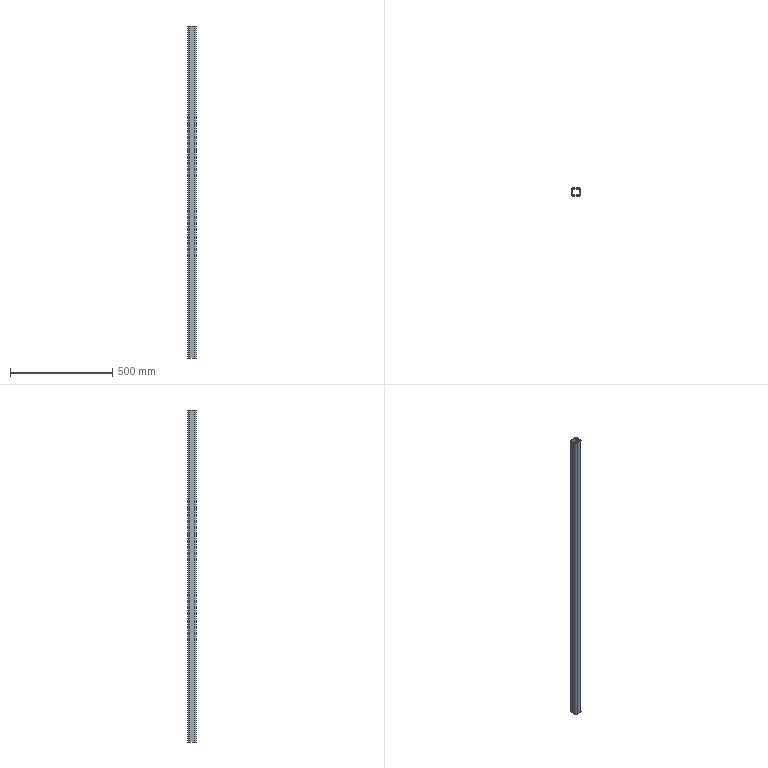Part | STEP file | 40 x 40 x 1700 | 1 solid | 18 faces | box 40 x 40 x 1620 mm | volume 866370 mm3 | plane 10 | cylinder 8 | commonest cylinder face diameters 8 x4 16 x4
STEP:
#1=CARTESIAN_POINT('',(32.,40.,1020.));
#2=VERTEX_POINT('',#1);
#3=CARTESIAN_POINT('',(8.,40.,1020.));
#4=VERTEX_POINT('',#3);
#5=CARTESIAN_POINT('',(32.,40.,1020.));
#6=DIRECTION('',(-1.,0.,0.));
#7=VECTOR('',#6,1000.);
#8=LINE('',#5,#7);
#9=EDGE_CURVE('',#2,#4,#8,.T.);
#10=ORIENTED_EDGE('',*,*,#9,.F.);
#11=CARTESIAN_POINT('',(32.,40.,-600.));
#12=VERTEX_POINT('',#11);
#13=CARTESIAN_POINT('',(32.,40.,600.));
#14=DIRECTION('',(0.,0.,1.));
#15=VECTOR('',#14,1000.);
#16=LINE('',#13,#15);
#17=EDGE_CURVE('',#12,#2,#16,.T.);
#18=ORIENTED_EDGE('',*,*,#17,.F.);
#19=CARTESIAN_POINT('',(8.,40.,-600.));
#20=VERTEX_POINT('',#19);
#21=CARTESIAN_POINT('',(32.,40.,-600.));
#22=DIRECTION('',(1.,0.,0.));
#23=VECTOR('',#22,1000.);
#24=LINE('',#21,#23);
#25=EDGE_CURVE('',#20,#12,#24,.T.);
#26=ORIENTED_EDGE('',*,*,#25,.F.);
#27=CARTESIAN_POINT('',(8.,40.,600.));
#28=DIRECTION('',(0.,0.,-1.));
#29=VECTOR('',#28,1000.);
#30=LINE('',#27,#29);
#31=EDGE_CURVE('',#4,#20,#30,.T.);
#32=ORIENTED_EDGE('',*,*,#31,.F.);
#33=EDGE_LOOP('',(#10,#18,#26,#32));
#34=FACE_OUTER_BOUND('',#33,.T.);
#35=CARTESIAN_POINT('',(32.,40.,600.));
#36=DIRECTION('',(0.,-1.,0.));
#37=DIRECTION('',(1.,0.,0.));
#38=AXIS2_PLACEMENT_3D('',#35,#36,#37);
#39=PLANE('',#38);
#40=ADVANCED_FACE('',(#34),#39,.F.);
#41=ORIENTED_EDGE('',*,*,#31,.T.);
#42=CARTESIAN_POINT('',(0.,32.,-600.));
#43=VERTEX_POINT('',#42);
#44=CARTESIAN_POINT('',(8.,32.,-600.));
#45=DIRECTION('',(0.,0.,1.));
#46=DIRECTION('',(-1.,0.,0.));
#47=AXIS2_PLACEMENT_3D('',#44,#45,#46);
#48=CIRCLE('',#47,8.);
#49=EDGE_CURVE('',#20,#43,#48,.T.);
#50=ORIENTED_EDGE('',*,*,#49,.T.);
#51=CARTESIAN_POINT('',(0.,32.,1020.));
#52=VERTEX_POINT('',#51);
#53=CARTESIAN_POINT('',(0.,32.,600.));
#54=DIRECTION('',(0.,0.,1.));
#55=VECTOR('',#54,1000.);
#56=LINE('',#53,#55);
#57=EDGE_CURVE('',#43,#52,#56,.T.);
#58=ORIENTED_EDGE('',*,*,#57,.T.);
#59=CARTESIAN_POINT('',(8.,32.,1020.));
#60=DIRECTION('',(0.,0.,-1.));
#61=DIRECTION('',(-1.,0.,0.));
#62=AXIS2_PLACEMENT_3D('',#59,#60,#61);
#63=CIRCLE('',#62,8.);
#64=EDGE_CURVE('',#52,#4,#63,.T.);
#65=ORIENTED_EDGE('',*,*,#64,.T.);
#66=EDGE_LOOP('',(#41,#50,#58,#65));
#67=FACE_OUTER_BOUND('',#66,.T.);
#68=CARTESIAN_POINT('',(8.,32.,600.));
#69=DIRECTION('',(0.,0.,-1.));
#70=DIRECTION('',(-1.,0.,0.));
#71=AXIS2_PLACEMENT_3D('',#68,#69,#70);
#72=CYLINDRICAL_SURFACE('',#71,8.);
#73=ADVANCED_FACE('',(#67),#72,.T.);
#74=CARTESIAN_POINT('',(8.,36.,1020.));
#75=VERTEX_POINT('',#74);
#76=CARTESIAN_POINT('',(32.,36.,1020.));
#77=VERTEX_POINT('',#76);
#78=CARTESIAN_POINT('',(32.,36.,1020.));
#79=DIRECTION('',(1.,0.,0.));
#80=VECTOR('',#79,1000.);
#81=LINE('',#78,#80);
#82=EDGE_CURVE('',#75,#77,#81,.T.);
#83=ORIENTED_EDGE('',*,*,#82,.T.);
#84=CARTESIAN_POINT('',(36.,32.,1020.));
#85=VERTEX_POINT('',#84);
#86=CARTESIAN_POINT('',(32.,32.,1020.));
#87=DIRECTION('',(0.,0.,-1.));
#88=DIRECTION('',(-1.,0.,0.));
#89=AXIS2_PLACEMENT_3D('',#86,#87,#88);
#90=CIRCLE('',#89,4.);
#91=EDGE_CURVE('',#77,#85,#90,.T.);
#92=ORIENTED_EDGE('',*,*,#91,.T.);
#93=CARTESIAN_POINT('',(36.,8.,1020.));
#94=VERTEX_POINT('',#93);
#95=CARTESIAN_POINT('',(36.,8.,1020.));
#96=DIRECTION('',(0.,-1.,0.));
#97=VECTOR('',#96,1000.);
#98=LINE('',#95,#97);
#99=EDGE_CURVE('',#85,#94,#98,.T.);
#100=ORIENTED_EDGE('',*,*,#99,.T.);
#101=CARTESIAN_POINT('',(32.,4.,1020.));
#102=VERTEX_POINT('',#101);
#103=CARTESIAN_POINT('',(32.,8.,1020.));
#104=DIRECTION('',(0.,0.,-1.));
#105=DIRECTION('',(-1.,0.,0.));
#106=AXIS2_PLACEMENT_3D('',#103,#104,#105);
#107=CIRCLE('',#106,4.);
#108=EDGE_CURVE('',#94,#102,#107,.T.);
#109=ORIENTED_EDGE('',*,*,#108,.T.);
#110=CARTESIAN_POINT('',(8.,4.,1020.));
#111=VERTEX_POINT('',#110);
#112=CARTESIAN_POINT('',(32.,4.,1020.));
#113=DIRECTION('',(-1.,0.,0.));
#114=VECTOR('',#113,1000.);
#115=LINE('',#112,#114);
#116=EDGE_CURVE('',#102,#111,#115,.T.);
#117=ORIENTED_EDGE('',*,*,#116,.T.);
#118=CARTESIAN_POINT('',(4.,8.,1020.));
#119=VERTEX_POINT('',#118);
#120=CARTESIAN_POINT('',(8.,8.,1020.));
#121=DIRECTION('',(0.,0.,-1.));
#122=DIRECTION('',(-1.,0.,0.));
#123=AXIS2_PLACEMENT_3D('',#120,#121,#122);
#124=CIRCLE('',#123,4.);
#125=EDGE_CURVE('',#111,#119,#124,.T.);
#126=ORIENTED_EDGE('',*,*,#125,.T.);
#127=CARTESIAN_POINT('',(4.,32.,1020.));
#128=VERTEX_POINT('',#127);
#129=CARTESIAN_POINT('',(4.,8.,1020.));
#130=DIRECTION('',(0.,1.,0.));
#131=VECTOR('',#130,1000.);
#132=LINE('',#129,#131);
#133=EDGE_CURVE('',#119,#128,#132,.T.);
#134=ORIENTED_EDGE('',*,*,#133,.T.);
#135=CARTESIAN_POINT('',(8.,32.,1020.));
#136=DIRECTION('',(0.,0.,-1.));
#137=DIRECTION('',(-1.,0.,0.));
#138=AXIS2_PLACEMENT_3D('',#135,#136,#137);
#139=CIRCLE('',#138,4.);
#140=EDGE_CURVE('',#128,#75,#139,.T.);
#141=ORIENTED_EDGE('',*,*,#140,.T.);
#142=EDGE_LOOP('',(#83,#92,#100,#109,#117,#126,#134,#141));
#143=FACE_BOUND('',#142,.T.);
#144=CARTESIAN_POINT('',(0.,8.,1020.));
#145=VERTEX_POINT('',#144);
#146=CARTESIAN_POINT('',(8.,0.,1020.));
#147=VERTEX_POINT('',#146);
#148=CARTESIAN_POINT('',(8.,8.,1020.));
#149=DIRECTION('',(0.,0.,1.));
#150=DIRECTION('',(-1.,0.,0.));
#151=AXIS2_PLACEMENT_3D('',#148,#149,#150);
#152=CIRCLE('',#151,8.);
#153=EDGE_CURVE('',#145,#147,#152,.T.);
#154=ORIENTED_EDGE('',*,*,#153,.T.);
#155=CARTESIAN_POINT('',(32.,0.,1020.));
#156=VERTEX_POINT('',#155);
#157=CARTESIAN_POINT('',(32.,0.,1020.));
#158=DIRECTION('',(1.,0.,0.));
#159=VECTOR('',#158,1000.);
#160=LINE('',#157,#159);
#161=EDGE_CURVE('',#147,#156,#160,.T.);
#162=ORIENTED_EDGE('',*,*,#161,.T.);
#163=CARTESIAN_POINT('',(40.,8.,1020.));
#164=VERTEX_POINT('',#163);
#165=CARTESIAN_POINT('',(32.,8.,1020.));
#166=DIRECTION('',(0.,0.,1.));
#167=DIRECTION('',(-1.,0.,0.));
#168=AXIS2_PLACEMENT_3D('',#165,#166,#167);
#169=CIRCLE('',#168,8.);
#170=EDGE_CURVE('',#156,#164,#169,.T.);
#171=ORIENTED_EDGE('',*,*,#170,.T.);
#172=CARTESIAN_POINT('',(40.,32.,1020.));
#173=VERTEX_POINT('',#172);
#174=CARTESIAN_POINT('',(40.,8.,1020.));
#175=DIRECTION('',(0.,1.,0.));
#176=VECTOR('',#175,1000.);
#177=LINE('',#174,#176);
#178=EDGE_CURVE('',#164,#173,#177,.T.);
#179=ORIENTED_EDGE('',*,*,#178,.T.);
#180=CARTESIAN_POINT('',(32.,32.,1020.));
#181=DIRECTION('',(0.,0.,1.));
#182=DIRECTION('',(-1.,0.,0.));
#183=AXIS2_PLACEMENT_3D('',#180,#181,#182);
#184=CIRCLE('',#183,8.);
#185=EDGE_CURVE('',#173,#2,#184,.T.);
#186=ORIENTED_EDGE('',*,*,#185,.T.);
#187=ORIENTED_EDGE('',*,*,#9,.T.);
#188=ORIENTED_EDGE('',*,*,#64,.F.);
#189=CARTESIAN_POINT('',(0.,8.,1020.));
#190=DIRECTION('',(0.,-1.,0.));
#191=VECTOR('',#190,1000.);
#192=LINE('',#189,#191);
#193=EDGE_CURVE('',#52,#145,#192,.T.);
#194=ORIENTED_EDGE('',*,*,#193,.T.);
#195=EDGE_LOOP('',(#154,#162,#171,#179,#186,#187,#188,#194));
#196=FACE_OUTER_BOUND('',#195,.T.);
#197=CARTESIAN_POINT('',(32.,8.,1020.));
#198=DIRECTION('',(0.,0.,1.));
#199=DIRECTION('',(1.,0.,0.));
#200=AXIS2_PLACEMENT_3D('',#197,#198,#199);
#201=PLANE('',#200);
#202=ADVANCED_FACE('',(#143,#196),#201,.T.);
#203=CARTESIAN_POINT('',(40.,32.,-600.));
#204=VERTEX_POINT('',#203);
#205=CARTESIAN_POINT('',(40.,32.,600.));
#206=DIRECTION('',(0.,0.,-1.));
#207=VECTOR('',#206,1000.);
#208=LINE('',#205,#207);
#209=EDGE_CURVE('',#173,#204,#208,.T.);
#210=ORIENTED_EDGE('',*,*,#209,.T.);
#211=CARTESIAN_POINT('',(32.,32.,-600.));
#212=DIRECTION('',(0.,0.,1.));
#213=DIRECTION('',(-1.,0.,0.));
#214=AXIS2_PLACEMENT_3D('',#211,#212,#213);
#215=CIRCLE('',#214,8.);
#216=EDGE_CURVE('',#204,#12,#215,.T.);
#217=ORIENTED_EDGE('',*,*,#216,.T.);
#218=ORIENTED_EDGE('',*,*,#17,.T.);
#219=ORIENTED_EDGE('',*,*,#185,.F.);
#220=EDGE_LOOP('',(#210,#217,#218,#219));
#221=FACE_OUTER_BOUND('',#220,.T.);
#222=CARTESIAN_POINT('',(32.,32.,600.));
#223=DIRECTION('',(0.,0.,-1.));
#224=DIRECTION('',(-1.,0.,0.));
#225=AXIS2_PLACEMENT_3D('',#222,#223,#224);
#226=CYLINDRICAL_SURFACE('',#225,8.);
#227=ADVANCED_FACE('',(#221),#226,.T.);
#228=CARTESIAN_POINT('',(32.,0.,-600.));
#229=VERTEX_POINT('',#228);
#230=CARTESIAN_POINT('',(40.,8.,-600.));
#231=VERTEX_POINT('',#230);
#232=CARTESIAN_POINT('',(32.,8.,-600.));
#233=DIRECTION('',(0.,0.,1.));
#234=DIRECTION('',(-1.,0.,0.));
#235=AXIS2_PLACEMENT_3D('',#232,#233,#234);
#236=CIRCLE('',#235,8.);
#237=EDGE_CURVE('',#229,#231,#236,.T.);
#238=ORIENTED_EDGE('',*,*,#237,.F.);
#239=CARTESIAN_POINT('',(8.,0.,-600.));
#240=VERTEX_POINT('',#239);
#241=CARTESIAN_POINT('',(32.,0.,-600.));
#242=DIRECTION('',(1.,0.,0.));
#243=VECTOR('',#242,1000.);
#244=LINE('',#241,#243);
#245=EDGE_CURVE('',#240,#229,#244,.T.);
#246=ORIENTED_EDGE('',*,*,#245,.F.);
#247=CARTESIAN_POINT('',(0.,8.,-600.));
#248=VERTEX_POINT('',#247);
#249=CARTESIAN_POINT('',(8.,8.,-600.));
#250=DIRECTION('',(0.,0.,1.));
#251=DIRECTION('',(-1.,0.,0.));
#252=AXIS2_PLACEMENT_3D('',#249,#250,#251);
#253=CIRCLE('',#252,8.);
#254=EDGE_CURVE('',#248,#240,#253,.T.);
#255=ORIENTED_EDGE('',*,*,#254,.F.);
#256=CARTESIAN_POINT('',(0.,32.,-600.));
#257=DIRECTION('',(0.,-1.,0.));
#258=VECTOR('',#257,1000.);
#259=LINE('',#256,#258);
#260=EDGE_CURVE('',#43,#248,#259,.T.);
#261=ORIENTED_EDGE('',*,*,#260,.F.);
#262=ORIENTED_EDGE('',*,*,#49,.F.);
#263=ORIENTED_EDGE('',*,*,#25,.T.);
#264=ORIENTED_EDGE('',*,*,#216,.F.);
#265=CARTESIAN_POINT('',(40.,32.,-600.));
#266=DIRECTION('',(0.,1.,0.));
#267=VECTOR('',#266,1000.);
#268=LINE('',#265,#267);
#269=EDGE_CURVE('',#231,#204,#268,.T.);
#270=ORIENTED_EDGE('',*,*,#269,.F.);
#271=EDGE_LOOP('',(#238,#246,#255,#261,#262,#263,#264,#270));
#272=FACE_OUTER_BOUND('',#271,.T.);
#273=CARTESIAN_POINT('',(8.,4.,-600.));
#274=VERTEX_POINT('',#273);
#275=CARTESIAN_POINT('',(4.,8.,-600.));
#276=VERTEX_POINT('',#275);
#277=CARTESIAN_POINT('',(8.,8.,-600.));
#278=DIRECTION('',(0.,0.,-1.));
#279=DIRECTION('',(-1.,0.,0.));
#280=AXIS2_PLACEMENT_3D('',#277,#278,#279);
#281=CIRCLE('',#280,4.);
#282=EDGE_CURVE('',#274,#276,#281,.T.);
#283=ORIENTED_EDGE('',*,*,#282,.F.);
#284=CARTESIAN_POINT('',(32.,4.,-600.));
#285=VERTEX_POINT('',#284);
#286=CARTESIAN_POINT('',(32.,4.,-600.));
#287=DIRECTION('',(-1.,0.,0.));
#288=VECTOR('',#287,1000.);
#289=LINE('',#286,#288);
#290=EDGE_CURVE('',#285,#274,#289,.T.);
#291=ORIENTED_EDGE('',*,*,#290,.F.);
#292=CARTESIAN_POINT('',(36.,8.,-600.));
#293=VERTEX_POINT('',#292);
#294=CARTESIAN_POINT('',(32.,8.,-600.));
#295=DIRECTION('',(0.,0.,-1.));
#296=DIRECTION('',(-1.,0.,0.));
#297=AXIS2_PLACEMENT_3D('',#294,#295,#296);
#298=CIRCLE('',#297,4.);
#299=EDGE_CURVE('',#293,#285,#298,.T.);
#300=ORIENTED_EDGE('',*,*,#299,.F.);
#301=CARTESIAN_POINT('',(36.,32.,-600.));
#302=VERTEX_POINT('',#301);
#303=CARTESIAN_POINT('',(36.,32.,-600.));
#304=DIRECTION('',(0.,-1.,0.));
#305=VECTOR('',#304,1000.);
#306=LINE('',#303,#305);
#307=EDGE_CURVE('',#302,#293,#306,.T.);
#308=ORIENTED_EDGE('',*,*,#307,.F.);
#309=CARTESIAN_POINT('',(32.,36.,-600.));
#310=VERTEX_POINT('',#309);
#311=CARTESIAN_POINT('',(32.,32.,-600.));
#312=DIRECTION('',(0.,0.,-1.));
#313=DIRECTION('',(-1.,0.,0.));
#314=AXIS2_PLACEMENT_3D('',#311,#312,#313);
#315=CIRCLE('',#314,4.);
#316=EDGE_CURVE('',#310,#302,#315,.T.);
#317=ORIENTED_EDGE('',*,*,#316,.F.);
#318=CARTESIAN_POINT('',(8.,36.,-600.));
#319=VERTEX_POINT('',#318);
#320=CARTESIAN_POINT('',(32.,36.,-600.));
#321=DIRECTION('',(1.,0.,0.));
#322=VECTOR('',#321,1000.);
#323=LINE('',#320,#322);
#324=EDGE_CURVE('',#319,#310,#323,.T.);
#325=ORIENTED_EDGE('',*,*,#324,.F.);
#326=CARTESIAN_POINT('',(4.,32.,-600.));
#327=VERTEX_POINT('',#326);
#328=CARTESIAN_POINT('',(8.,32.,-600.));
#329=DIRECTION('',(0.,0.,-1.));
#330=DIRECTION('',(-1.,0.,0.));
#331=AXIS2_PLACEMENT_3D('',#328,#329,#330);
#332=CIRCLE('',#331,4.);
#333=EDGE_CURVE('',#327,#319,#332,.T.);
#334=ORIENTED_EDGE('',*,*,#333,.F.);
#335=CARTESIAN_POINT('',(4.,32.,-600.));
#336=DIRECTION('',(0.,1.,0.));
#337=VECTOR('',#336,1000.);
#338=LINE('',#335,#337);
#339=EDGE_CURVE('',#276,#327,#338,.T.);
#340=ORIENTED_EDGE('',*,*,#339,.F.);
#341=EDGE_LOOP('',(#283,#291,#300,#308,#317,#325,#334,#340));
#342=FACE_BOUND('',#341,.T.);
#343=CARTESIAN_POINT('',(32.,32.,-600.));
#344=DIRECTION('',(0.,0.,1.));
#345=DIRECTION('',(1.,0.,0.));
#346=AXIS2_PLACEMENT_3D('',#343,#344,#345);
#347=PLANE('',#346);
#348=ADVANCED_FACE('',(#272,#342),#347,.F.);
#349=ORIENTED_EDGE('',*,*,#193,.F.);
#350=ORIENTED_EDGE('',*,*,#57,.F.);
#351=ORIENTED_EDGE('',*,*,#260,.T.);
#352=CARTESIAN_POINT('',(0.,8.,600.));
#353=DIRECTION('',(0.,0.,-1.));
#354=VECTOR('',#353,1000.);
#355=LINE('',#352,#354);
#356=EDGE_CURVE('',#145,#248,#355,.T.);
#357=ORIENTED_EDGE('',*,*,#356,.F.);
#358=EDGE_LOOP('',(#349,#350,#351,#357));
#359=FACE_OUTER_BOUND('',#358,.T.);
#360=CARTESIAN_POINT('',(0.,8.,600.));
#361=DIRECTION('',(1.,0.,0.));
#362=DIRECTION('',(0.,1.,0.));
#363=AXIS2_PLACEMENT_3D('',#360,#361,#362);
#364=PLANE('',#363);
#365=ADVANCED_FACE('',(#359),#364,.F.);
#366=ORIENTED_EDGE('',*,*,#91,.F.);
#367=CARTESIAN_POINT('',(32.,36.,600.));
#368=DIRECTION('',(0.,0.,1.));
#369=VECTOR('',#368,1000.);
#370=LINE('',#367,#369);
#371=EDGE_CURVE('',#310,#77,#370,.T.);
#372=ORIENTED_EDGE('',*,*,#371,.F.);
#373=ORIENTED_EDGE('',*,*,#316,.T.);
#374=CARTESIAN_POINT('',(36.,32.,600.));
#375=DIRECTION('',(0.,0.,-1.));
#376=VECTOR('',#375,1000.);
#377=LINE('',#374,#376);
#378=EDGE_CURVE('',#85,#302,#377,.T.);
#379=ORIENTED_EDGE('',*,*,#378,.F.);
#380=EDGE_LOOP('',(#366,#372,#373,#379));
#381=FACE_OUTER_BOUND('',#380,.T.);
#382=CARTESIAN_POINT('',(32.,32.,600.));
#383=DIRECTION('',(0.,0.,-1.));
#384=DIRECTION('',(-1.,0.,0.));
#385=AXIS2_PLACEMENT_3D('',#382,#383,#384);
#386=CYLINDRICAL_SURFACE('',#385,4.);
#387=ADVANCED_FACE('',(#381),#386,.F.);
#388=CARTESIAN_POINT('',(8.,36.,600.));
#389=DIRECTION('',(0.,0.,-1.));
#390=VECTOR('',#389,1000.);
#391=LINE('',#388,#390);
#392=EDGE_CURVE('',#75,#319,#391,.T.);
#393=ORIENTED_EDGE('',*,*,#392,.T.);
#394=ORIENTED_EDGE('',*,*,#324,.T.);
#395=ORIENTED_EDGE('',*,*,#371,.T.);
#396=ORIENTED_EDGE('',*,*,#82,.F.);
#397=EDGE_LOOP('',(#393,#394,#395,#396));
#398=FACE_OUTER_BOUND('',#397,.T.);
#399=CARTESIAN_POINT('',(32.,36.,600.));
#400=DIRECTION('',(0.,-1.,0.));
#401=DIRECTION('',(0.,0.,-1.));
#402=AXIS2_PLACEMENT_3D('',#399,#400,#401);
#403=PLANE('',#402);
#404=ADVANCED_FACE('',(#398),#403,.T.);
#405=ORIENTED_EDGE('',*,*,#140,.F.);
#406=CARTESIAN_POINT('',(4.,32.,600.));
#407=DIRECTION('',(0.,0.,1.));
#408=VECTOR('',#407,1000.);
#409=LINE('',#406,#408);
#410=EDGE_CURVE('',#327,#128,#409,.T.);
#411=ORIENTED_EDGE('',*,*,#410,.F.);
#412=ORIENTED_EDGE('',*,*,#333,.T.);
#413=ORIENTED_EDGE('',*,*,#392,.F.);
#414=EDGE_LOOP('',(#405,#411,#412,#413));
#415=FACE_OUTER_BOUND('',#414,.T.);
#416=CARTESIAN_POINT('',(8.,32.,600.));
#417=DIRECTION('',(0.,0.,-1.));
#418=DIRECTION('',(-1.,0.,0.));
#419=AXIS2_PLACEMENT_3D('',#416,#417,#418);
#420=CYLINDRICAL_SURFACE('',#419,4.);
#421=ADVANCED_FACE('',(#415),#420,.F.);
#422=CARTESIAN_POINT('',(4.,8.,600.));
#423=DIRECTION('',(0.,0.,-1.));
#424=VECTOR('',#423,1000.);
#425=LINE('',#422,#424);
#426=EDGE_CURVE('',#119,#276,#425,.T.);
#427=ORIENTED_EDGE('',*,*,#426,.T.);
#428=ORIENTED_EDGE('',*,*,#339,.T.);
#429=ORIENTED_EDGE('',*,*,#410,.T.);
#430=ORIENTED_EDGE('',*,*,#133,.F.);
#431=EDGE_LOOP('',(#427,#428,#429,#430));
#432=FACE_OUTER_BOUND('',#431,.T.);
#433=CARTESIAN_POINT('',(4.,8.,600.));
#434=DIRECTION('',(1.,0.,0.));
#435=DIRECTION('',(0.,1.,0.));
#436=AXIS2_PLACEMENT_3D('',#433,#434,#435);
#437=PLANE('',#436);
#438=ADVANCED_FACE('',(#432),#437,.T.);
#439=ORIENTED_EDGE('',*,*,#125,.F.);
#440=CARTESIAN_POINT('',(8.,4.,600.));
#441=DIRECTION('',(0.,0.,1.));
#442=VECTOR('',#441,1000.);
#443=LINE('',#440,#442);
#444=EDGE_CURVE('',#274,#111,#443,.T.);
#445=ORIENTED_EDGE('',*,*,#444,.F.);
#446=ORIENTED_EDGE('',*,*,#282,.T.);
#447=ORIENTED_EDGE('',*,*,#426,.F.);
#448=EDGE_LOOP('',(#439,#445,#446,#447));
#449=FACE_OUTER_BOUND('',#448,.T.);
#450=CARTESIAN_POINT('',(8.,8.,600.));
#451=DIRECTION('',(0.,0.,-1.));
#452=DIRECTION('',(-1.,0.,0.));
#453=AXIS2_PLACEMENT_3D('',#450,#451,#452);
#454=CYLINDRICAL_SURFACE('',#453,4.);
#455=ADVANCED_FACE('',(#449),#454,.F.);
#456=CARTESIAN_POINT('',(32.,4.,600.));
#457=DIRECTION('',(0.,0.,-1.));
#458=VECTOR('',#457,1000.);
#459=LINE('',#456,#458);
#460=EDGE_CURVE('',#102,#285,#459,.T.);
#461=ORIENTED_EDGE('',*,*,#460,.T.);
#462=ORIENTED_EDGE('',*,*,#290,.T.);
#463=ORIENTED_EDGE('',*,*,#444,.T.);
#464=ORIENTED_EDGE('',*,*,#116,.F.);
#465=EDGE_LOOP('',(#461,#462,#463,#464));
#466=FACE_OUTER_BOUND('',#465,.T.);
#467=CARTESIAN_POINT('',(8.,4.,600.));
#468=DIRECTION('',(0.,1.,0.));
#469=DIRECTION('',(-1.,0.,0.));
#470=AXIS2_PLACEMENT_3D('',#467,#468,#469);
#471=PLANE('',#470);
#472=ADVANCED_FACE('',(#466),#471,.T.);
#473=ORIENTED_EDGE('',*,*,#108,.F.);
#474=CARTESIAN_POINT('',(36.,8.,600.));
#475=DIRECTION('',(0.,0.,1.));
#476=VECTOR('',#475,1000.);
#477=LINE('',#474,#476);
#478=EDGE_CURVE('',#293,#94,#477,.T.);
#479=ORIENTED_EDGE('',*,*,#478,.F.);
#480=ORIENTED_EDGE('',*,*,#299,.T.);
#481=ORIENTED_EDGE('',*,*,#460,.F.);
#482=EDGE_LOOP('',(#473,#479,#480,#481));
#483=FACE_OUTER_BOUND('',#482,.T.);
#484=CARTESIAN_POINT('',(32.,8.,600.));
#485=DIRECTION('',(0.,0.,-1.));
#486=DIRECTION('',(-1.,0.,0.));
#487=AXIS2_PLACEMENT_3D('',#484,#485,#486);
#488=CYLINDRICAL_SURFACE('',#487,4.);
#489=ADVANCED_FACE('',(#483),#488,.F.);
#490=ORIENTED_EDGE('',*,*,#378,.T.);
#491=ORIENTED_EDGE('',*,*,#307,.T.);
#492=ORIENTED_EDGE('',*,*,#478,.T.);
#493=ORIENTED_EDGE('',*,*,#99,.F.);
#494=EDGE_LOOP('',(#490,#491,#492,#493));
#495=FACE_OUTER_BOUND('',#494,.T.);
#496=CARTESIAN_POINT('',(36.,32.,600.));
#497=DIRECTION('',(-1.,0.,0.));
#498=DIRECTION('',(0.,0.,1.));
#499=AXIS2_PLACEMENT_3D('',#496,#497,#498);
#500=PLANE('',#499);
#501=ADVANCED_FACE('',(#495),#500,.T.);
#502=ORIENTED_EDGE('',*,*,#161,.F.);
#503=CARTESIAN_POINT('',(8.,0.,600.));
#504=DIRECTION('',(0.,0.,1.));
#505=VECTOR('',#504,1000.);
#506=LINE('',#503,#505);
#507=EDGE_CURVE('',#240,#147,#506,.T.);
#508=ORIENTED_EDGE('',*,*,#507,.F.);
#509=ORIENTED_EDGE('',*,*,#245,.T.);
#510=CARTESIAN_POINT('',(32.,0.,600.));
#511=DIRECTION('',(0.,0.,-1.));
#512=VECTOR('',#511,1000.);
#513=LINE('',#510,#512);
#514=EDGE_CURVE('',#156,#229,#513,.T.);
#515=ORIENTED_EDGE('',*,*,#514,.F.);
#516=EDGE_LOOP('',(#502,#508,#509,#515));
#517=FACE_OUTER_BOUND('',#516,.T.);
#518=CARTESIAN_POINT('',(8.,0.,600.));
#519=DIRECTION('',(0.,1.,0.));
#520=DIRECTION('',(-1.,0.,0.));
#521=AXIS2_PLACEMENT_3D('',#518,#519,#520);
#522=PLANE('',#521);
#523=ADVANCED_FACE('',(#517),#522,.F.);
#524=ORIENTED_EDGE('',*,*,#356,.T.);
#525=ORIENTED_EDGE('',*,*,#254,.T.);
#526=ORIENTED_EDGE('',*,*,#507,.T.);
#527=ORIENTED_EDGE('',*,*,#153,.F.);
#528=EDGE_LOOP('',(#524,#525,#526,#527));
#529=FACE_OUTER_BOUND('',#528,.T.);
#530=CARTESIAN_POINT('',(8.,8.,600.));
#531=DIRECTION('',(0.,0.,-1.));
#532=DIRECTION('',(-1.,0.,0.));
#533=AXIS2_PLACEMENT_3D('',#530,#531,#532);
#534=CYLINDRICAL_SURFACE('',#533,8.);
#535=ADVANCED_FACE('',(#529),#534,.T.);
#536=ORIENTED_EDGE('',*,*,#178,.F.);
#537=CARTESIAN_POINT('',(40.,8.,600.));
#538=DIRECTION('',(0.,0.,1.));
#539=VECTOR('',#538,1000.);
#540=LINE('',#537,#539);
#541=EDGE_CURVE('',#231,#164,#540,.T.);
#542=ORIENTED_EDGE('',*,*,#541,.F.);
#543=ORIENTED_EDGE('',*,*,#269,.T.);
#544=ORIENTED_EDGE('',*,*,#209,.F.);
#545=EDGE_LOOP('',(#536,#542,#543,#544));
#546=FACE_OUTER_BOUND('',#545,.T.);
#547=CARTESIAN_POINT('',(40.,32.,600.));
#548=DIRECTION('',(-1.,0.,0.));
#549=DIRECTION('',(0.,-1.,0.));
#550=AXIS2_PLACEMENT_3D('',#547,#548,#549);
#551=PLANE('',#550);
#552=ADVANCED_FACE('',(#546),#551,.F.);
#553=ORIENTED_EDGE('',*,*,#514,.T.);
#554=ORIENTED_EDGE('',*,*,#237,.T.);
#555=ORIENTED_EDGE('',*,*,#541,.T.);
#556=ORIENTED_EDGE('',*,*,#170,.F.);
#557=EDGE_LOOP('',(#553,#554,#555,#556));
#558=FACE_OUTER_BOUND('',#557,.T.);
#559=CARTESIAN_POINT('',(32.,8.,600.));
#560=DIRECTION('',(0.,0.,-1.));
#561=DIRECTION('',(-1.,0.,0.));
#562=AXIS2_PLACEMENT_3D('',#559,#560,#561);
#563=CYLINDRICAL_SURFACE('',#562,8.);
#564=ADVANCED_FACE('',(#558),#563,.T.);
#565=CLOSED_SHELL('',(#40,#73,#202,#227,#348,#365,#387,#404,#421,#438,#455,#472,#489,#501,#523,#535,#552,#564));
#566=MANIFOLD_SOLID_BREP('',#565);
#567=CARTESIAN_POINT('',(0.,0.,0.));
#568=DIRECTION('',(0.,0.,1.));
#569=DIRECTION('',(1.,0.,0.));
#570=AXIS2_PLACEMENT_3D('',#567,#568,#569);
#571=(LENGTH_UNIT()NAMED_UNIT(*)SI_UNIT(.MILLI.,.METRE.));
#572=UNCERTAINTY_MEASURE_WITH_UNIT(LENGTH_MEASURE(0.00001),#571,'','');
#573=(NAMED_UNIT(*)PLANE_ANGLE_UNIT()SI_UNIT($,.RADIAN.));
#574=(NAMED_UNIT(*)SI_UNIT($,.STERADIAN.)SOLID_ANGLE_UNIT());
#575=(GEOMETRIC_REPRESENTATION_CONTEXT(3)GLOBAL_UNCERTAINTY_ASSIGNED_CONTEXT((#572))GLOBAL_UNIT_ASSIGNED_CONTEXT((#571,#573,#574))REPRESENTATION_CONTEXT('',''));
#576=ADVANCED_BREP_SHAPE_REPRESENTATION('',(#566,#570),#575);